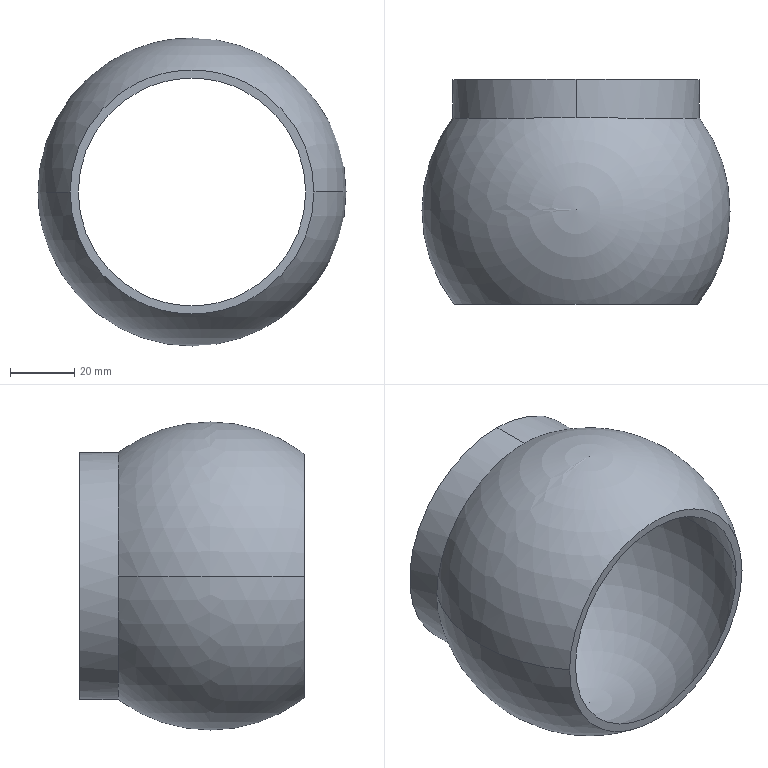Part | SolidWorks | features Revolution 1, Shell 1 | 1 solid | 10 faces | box 96 x 70 x 96 mm | volume 39871 mm3 | sphere 4 | cylinder 4 | plane 2 | commonest cylinder face diameters 73 x2 77 x2
STEP:
#1=CARTESIAN_POINT('',(35.433,-70.,0.));
#2=VERTEX_POINT('',#1);
#3=CARTESIAN_POINT('',(-35.433,-70.,0.));
#4=VERTEX_POINT('',#3);
#5=CARTESIAN_POINT('',(0.,-70.,0.));
#6=DIRECTION('',(0.,1.,0.));
#7=DIRECTION('',(0.,0.,-1.));
#8=AXIS2_PLACEMENT_3D('',#5,#6,#7);
#9=CIRCLE('',#8,35.433);
#10=EDGE_CURVE('',#2,#4,#9,.T.);
#11=ORIENTED_EDGE('',*,*,#10,.F.);
#12=CARTESIAN_POINT('',(36.5,-12.671,0.));
#13=VERTEX_POINT('',#12);
#14=CARTESIAN_POINT('',(0.,-40.666,0.));
#15=DIRECTION('',(0.,0.,1.));
#16=DIRECTION('',(1.,0.,0.));
#17=AXIS2_PLACEMENT_3D('',#14,#15,#16);
#18=CIRCLE('',#17,46.);
#19=EDGE_CURVE('',#2,#13,#18,.T.);
#20=ORIENTED_EDGE('',*,*,#19,.T.);
#21=CARTESIAN_POINT('',(0.,-12.671,-36.5));
#22=VERTEX_POINT('',#21);
#23=CARTESIAN_POINT('',(0.,-12.671,0.));
#24=DIRECTION('',(0.,1.,0.));
#25=DIRECTION('',(0.,0.,-1.));
#26=AXIS2_PLACEMENT_3D('',#23,#24,#25);
#27=CIRCLE('',#26,36.5);
#28=EDGE_CURVE('',#13,#22,#27,.T.);
#29=ORIENTED_EDGE('',*,*,#28,.T.);
#30=CARTESIAN_POINT('',(-36.5,-12.671,0.));
#31=VERTEX_POINT('',#30);
#32=CARTESIAN_POINT('',(0.,-12.671,0.));
#33=DIRECTION('',(0.,1.,0.));
#34=DIRECTION('',(0.,0.,-1.));
#35=AXIS2_PLACEMENT_3D('',#32,#33,#34);
#36=CIRCLE('',#35,36.5);
#37=EDGE_CURVE('',#22,#31,#36,.T.);
#38=ORIENTED_EDGE('',*,*,#37,.T.);
#39=CARTESIAN_POINT('',(0.,-40.666,0.));
#40=DIRECTION('',(0.,0.,-1.));
#41=DIRECTION('',(-1.,0.,0.));
#42=AXIS2_PLACEMENT_3D('',#39,#40,#41);
#43=CIRCLE('',#42,46.);
#44=EDGE_CURVE('',#4,#31,#43,.T.);
#45=ORIENTED_EDGE('',*,*,#44,.F.);
#46=EDGE_LOOP('',(#11,#20,#29,#38,#45));
#47=FACE_OUTER_BOUND('',#46,.T.);
#48=CARTESIAN_POINT('',(0.,-40.666,0.));
#49=DIRECTION('',(0.,0.,1.));
#50=DIRECTION('',(-1.,0.,0.));
#51=AXIS2_PLACEMENT_3D('',#48,#49,#50);
#52=SPHERICAL_SURFACE('',#51,46.);
#53=ADVANCED_FACE('',(#47),#52,.F.);
#54=ORIENTED_EDGE('',*,*,#37,.F.);
#55=CARTESIAN_POINT('',(0.,0.,-36.5));
#56=VERTEX_POINT('',#55);
#57=CARTESIAN_POINT('',(0.,0.,-36.5));
#58=DIRECTION('',(0.,1.,0.));
#59=VECTOR('',#58,1000.);
#60=LINE('',#57,#59);
#61=EDGE_CURVE('',#22,#56,#60,.T.);
#62=ORIENTED_EDGE('',*,*,#61,.T.);
#63=CARTESIAN_POINT('',(0.,0.,36.5));
#64=VERTEX_POINT('',#63);
#65=CARTESIAN_POINT('',(0.,0.,0.));
#66=DIRECTION('',(0.,1.,0.));
#67=DIRECTION('',(0.,0.,1.));
#68=AXIS2_PLACEMENT_3D('',#65,#66,#67);
#69=CIRCLE('',#68,36.5);
#70=EDGE_CURVE('',#56,#64,#69,.T.);
#71=ORIENTED_EDGE('',*,*,#70,.T.);
#72=CARTESIAN_POINT('',(0.,-12.671,36.5));
#73=VERTEX_POINT('',#72);
#74=CARTESIAN_POINT('',(0.,0.,36.5));
#75=DIRECTION('',(0.,1.,0.));
#76=VECTOR('',#75,1000.);
#77=LINE('',#74,#76);
#78=EDGE_CURVE('',#73,#64,#77,.T.);
#79=ORIENTED_EDGE('',*,*,#78,.F.);
#80=CARTESIAN_POINT('',(0.,-12.671,0.));
#81=DIRECTION('',(0.,1.,0.));
#82=DIRECTION('',(0.,0.,-1.));
#83=AXIS2_PLACEMENT_3D('',#80,#81,#82);
#84=CIRCLE('',#83,36.5);
#85=EDGE_CURVE('',#31,#73,#84,.T.);
#86=ORIENTED_EDGE('',*,*,#85,.F.);
#87=EDGE_LOOP('',(#54,#62,#71,#79,#86));
#88=FACE_OUTER_BOUND('',#87,.T.);
#89=CARTESIAN_POINT('',(0.,0.,0.));
#90=DIRECTION('',(0.,1.,0.));
#91=DIRECTION('',(0.,0.,1.));
#92=AXIS2_PLACEMENT_3D('',#89,#90,#91);
#93=CYLINDRICAL_SURFACE('',#92,36.5);
#94=ADVANCED_FACE('',(#88),#93,.F.);
#95=CARTESIAN_POINT('',(-37.994,-70.,0.));
#96=VERTEX_POINT('',#95);
#97=CARTESIAN_POINT('',(37.994,-70.,0.));
#98=VERTEX_POINT('',#97);
#99=CARTESIAN_POINT('',(0.,-70.,0.));
#100=DIRECTION('',(0.,1.,0.));
#101=DIRECTION('',(0.,0.,1.));
#102=AXIS2_PLACEMENT_3D('',#99,#100,#101);
#103=CIRCLE('',#102,37.994);
#104=EDGE_CURVE('',#96,#98,#103,.T.);
#105=ORIENTED_EDGE('',*,*,#104,.T.);
#106=CARTESIAN_POINT('',(38.5,-12.,0.));
#107=VERTEX_POINT('',#106);
#108=CARTESIAN_POINT('',(0.,-40.666,0.));
#109=DIRECTION('',(0.,0.,1.));
#110=DIRECTION('',(1.,0.,0.));
#111=AXIS2_PLACEMENT_3D('',#108,#109,#110);
#112=CIRCLE('',#111,48.);
#113=EDGE_CURVE('',#98,#107,#112,.T.);
#114=ORIENTED_EDGE('',*,*,#113,.T.);
#115=CARTESIAN_POINT('',(0.,-12.,38.5));
#116=VERTEX_POINT('',#115);
#117=CARTESIAN_POINT('',(0.,-12.,0.));
#118=DIRECTION('',(0.,1.,0.));
#119=DIRECTION('',(0.,0.,1.));
#120=AXIS2_PLACEMENT_3D('',#117,#118,#119);
#121=CIRCLE('',#120,38.5);
#122=EDGE_CURVE('',#116,#107,#121,.T.);
#123=ORIENTED_EDGE('',*,*,#122,.F.);
#124=CARTESIAN_POINT('',(-38.5,-12.,0.));
#125=VERTEX_POINT('',#124);
#126=CARTESIAN_POINT('',(0.,-12.,0.));
#127=DIRECTION('',(0.,1.,0.));
#128=DIRECTION('',(0.,0.,1.));
#129=AXIS2_PLACEMENT_3D('',#126,#127,#128);
#130=CIRCLE('',#129,38.5);
#131=EDGE_CURVE('',#125,#116,#130,.T.);
#132=ORIENTED_EDGE('',*,*,#131,.F.);
#133=CARTESIAN_POINT('',(0.,-40.666,0.));
#134=DIRECTION('',(0.,0.,-1.));
#135=DIRECTION('',(-1.,0.,0.));
#136=AXIS2_PLACEMENT_3D('',#133,#134,#135);
#137=CIRCLE('',#136,48.);
#138=EDGE_CURVE('',#96,#125,#137,.T.);
#139=ORIENTED_EDGE('',*,*,#138,.F.);
#140=EDGE_LOOP('',(#105,#114,#123,#132,#139));
#141=FACE_OUTER_BOUND('',#140,.T.);
#142=CARTESIAN_POINT('',(0.,-40.666,0.));
#143=DIRECTION('',(0.,0.,1.));
#144=DIRECTION('',(-1.,0.,0.));
#145=AXIS2_PLACEMENT_3D('',#142,#143,#144);
#146=SPHERICAL_SURFACE('',#145,48.);
#147=ADVANCED_FACE('',(#141),#146,.T.);
#148=ORIENTED_EDGE('',*,*,#122,.T.);
#149=CARTESIAN_POINT('',(0.,-12.,-38.5));
#150=VERTEX_POINT('',#149);
#151=CARTESIAN_POINT('',(0.,-12.,0.));
#152=DIRECTION('',(0.,1.,0.));
#153=DIRECTION('',(0.,0.,1.));
#154=AXIS2_PLACEMENT_3D('',#151,#152,#153);
#155=CIRCLE('',#154,38.5);
#156=EDGE_CURVE('',#107,#150,#155,.T.);
#157=ORIENTED_EDGE('',*,*,#156,.T.);
#158=CARTESIAN_POINT('',(0.,0.,-38.5));
#159=VERTEX_POINT('',#158);
#160=CARTESIAN_POINT('',(0.,0.,-38.5));
#161=DIRECTION('',(0.,1.,0.));
#162=VECTOR('',#161,1000.);
#163=LINE('',#160,#162);
#164=EDGE_CURVE('',#150,#159,#163,.T.);
#165=ORIENTED_EDGE('',*,*,#164,.T.);
#166=CARTESIAN_POINT('',(0.,0.,38.5));
#167=VERTEX_POINT('',#166);
#168=CARTESIAN_POINT('',(0.,0.,0.));
#169=DIRECTION('',(0.,1.,0.));
#170=DIRECTION('',(0.,0.,1.));
#171=AXIS2_PLACEMENT_3D('',#168,#169,#170);
#172=CIRCLE('',#171,38.5);
#173=EDGE_CURVE('',#167,#159,#172,.T.);
#174=ORIENTED_EDGE('',*,*,#173,.F.);
#175=CARTESIAN_POINT('',(0.,0.,38.5));
#176=DIRECTION('',(0.,1.,0.));
#177=VECTOR('',#176,1000.);
#178=LINE('',#175,#177);
#179=EDGE_CURVE('',#116,#167,#178,.T.);
#180=ORIENTED_EDGE('',*,*,#179,.F.);
#181=EDGE_LOOP('',(#148,#157,#165,#174,#180));
#182=FACE_OUTER_BOUND('',#181,.T.);
#183=CARTESIAN_POINT('',(0.,0.,0.));
#184=DIRECTION('',(0.,1.,0.));
#185=DIRECTION('',(0.,0.,1.));
#186=AXIS2_PLACEMENT_3D('',#183,#184,#185);
#187=CYLINDRICAL_SURFACE('',#186,38.5);
#188=ADVANCED_FACE('',(#182),#187,.T.);
#189=ORIENTED_EDGE('',*,*,#104,.F.);
#190=CARTESIAN_POINT('',(0.,-70.,0.));
#191=DIRECTION('',(0.,1.,0.));
#192=DIRECTION('',(0.,0.,1.));
#193=AXIS2_PLACEMENT_3D('',#190,#191,#192);
#194=CIRCLE('',#193,37.994);
#195=EDGE_CURVE('',#98,#96,#194,.T.);
#196=ORIENTED_EDGE('',*,*,#195,.F.);
#197=EDGE_LOOP('',(#189,#196));
#198=FACE_OUTER_BOUND('',#197,.T.);
#199=CARTESIAN_POINT('',(0.,-70.,0.));
#200=DIRECTION('',(0.,1.,0.));
#201=DIRECTION('',(0.,0.,-1.));
#202=AXIS2_PLACEMENT_3D('',#199,#200,#201);
#203=CIRCLE('',#202,35.433);
#204=EDGE_CURVE('',#4,#2,#203,.T.);
#205=ORIENTED_EDGE('',*,*,#204,.T.);
#206=ORIENTED_EDGE('',*,*,#10,.T.);
#207=EDGE_LOOP('',(#205,#206));
#208=FACE_BOUND('',#207,.T.);
#209=CARTESIAN_POINT('',(-37.994,-70.,0.));
#210=DIRECTION('',(0.,-1.,0.));
#211=DIRECTION('',(0.,0.,-1.));
#212=AXIS2_PLACEMENT_3D('',#209,#210,#211);
#213=PLANE('',#212);
#214=ADVANCED_FACE('',(#198,#208),#213,.T.);
#215=CARTESIAN_POINT('',(0.,0.,0.));
#216=DIRECTION('',(0.,1.,0.));
#217=DIRECTION('',(0.,0.,1.));
#218=AXIS2_PLACEMENT_3D('',#215,#216,#217);
#219=CIRCLE('',#218,36.5);
#220=EDGE_CURVE('',#64,#56,#219,.T.);
#221=ORIENTED_EDGE('',*,*,#220,.F.);
#222=ORIENTED_EDGE('',*,*,#70,.F.);
#223=EDGE_LOOP('',(#221,#222));
#224=FACE_BOUND('',#223,.T.);
#225=ORIENTED_EDGE('',*,*,#173,.T.);
#226=CARTESIAN_POINT('',(0.,0.,0.));
#227=DIRECTION('',(0.,1.,0.));
#228=DIRECTION('',(0.,0.,1.));
#229=AXIS2_PLACEMENT_3D('',#226,#227,#228);
#230=CIRCLE('',#229,38.5);
#231=EDGE_CURVE('',#159,#167,#230,.T.);
#232=ORIENTED_EDGE('',*,*,#231,.T.);
#233=EDGE_LOOP('',(#225,#232));
#234=FACE_OUTER_BOUND('',#233,.T.);
#235=CARTESIAN_POINT('',(0.,0.,0.));
#236=DIRECTION('',(0.,1.,0.));
#237=DIRECTION('',(0.,0.,1.));
#238=AXIS2_PLACEMENT_3D('',#235,#236,#237);
#239=PLANE('',#238);
#240=ADVANCED_FACE('',(#224,#234),#239,.T.);
#241=ORIENTED_EDGE('',*,*,#164,.F.);
#242=CARTESIAN_POINT('',(0.,-12.,0.));
#243=DIRECTION('',(0.,1.,0.));
#244=DIRECTION('',(0.,0.,1.));
#245=AXIS2_PLACEMENT_3D('',#242,#243,#244);
#246=CIRCLE('',#245,38.5);
#247=EDGE_CURVE('',#150,#125,#246,.T.);
#248=ORIENTED_EDGE('',*,*,#247,.T.);
#249=ORIENTED_EDGE('',*,*,#131,.T.);
#250=ORIENTED_EDGE('',*,*,#179,.T.);
#251=ORIENTED_EDGE('',*,*,#231,.F.);
#252=EDGE_LOOP('',(#241,#248,#249,#250,#251));
#253=FACE_OUTER_BOUND('',#252,.T.);
#254=CARTESIAN_POINT('',(0.,0.,0.));
#255=DIRECTION('',(0.,1.,0.));
#256=DIRECTION('',(0.,0.,1.));
#257=AXIS2_PLACEMENT_3D('',#254,#255,#256);
#258=CYLINDRICAL_SURFACE('',#257,38.5);
#259=ADVANCED_FACE('',(#253),#258,.T.);
#260=ORIENTED_EDGE('',*,*,#113,.F.);
#261=ORIENTED_EDGE('',*,*,#195,.T.);
#262=ORIENTED_EDGE('',*,*,#138,.T.);
#263=ORIENTED_EDGE('',*,*,#247,.F.);
#264=ORIENTED_EDGE('',*,*,#156,.F.);
#265=EDGE_LOOP('',(#260,#261,#262,#263,#264));
#266=FACE_OUTER_BOUND('',#265,.T.);
#267=CARTESIAN_POINT('',(0.,-40.666,0.));
#268=DIRECTION('',(0.,0.,1.));
#269=DIRECTION('',(-1.,0.,0.));
#270=AXIS2_PLACEMENT_3D('',#267,#268,#269);
#271=SPHERICAL_SURFACE('',#270,48.);
#272=ADVANCED_FACE('',(#266),#271,.T.);
#273=ORIENTED_EDGE('',*,*,#61,.F.);
#274=ORIENTED_EDGE('',*,*,#28,.F.);
#275=CARTESIAN_POINT('',(0.,-12.671,0.));
#276=DIRECTION('',(0.,1.,0.));
#277=DIRECTION('',(0.,0.,-1.));
#278=AXIS2_PLACEMENT_3D('',#275,#276,#277);
#279=CIRCLE('',#278,36.5);
#280=EDGE_CURVE('',#73,#13,#279,.T.);
#281=ORIENTED_EDGE('',*,*,#280,.F.);
#282=ORIENTED_EDGE('',*,*,#78,.T.);
#283=ORIENTED_EDGE('',*,*,#220,.T.);
#284=EDGE_LOOP('',(#273,#274,#281,#282,#283));
#285=FACE_OUTER_BOUND('',#284,.T.);
#286=CARTESIAN_POINT('',(0.,0.,0.));
#287=DIRECTION('',(0.,1.,0.));
#288=DIRECTION('',(0.,0.,1.));
#289=AXIS2_PLACEMENT_3D('',#286,#287,#288);
#290=CYLINDRICAL_SURFACE('',#289,36.5);
#291=ADVANCED_FACE('',(#285),#290,.F.);
#292=ORIENTED_EDGE('',*,*,#19,.F.);
#293=ORIENTED_EDGE('',*,*,#204,.F.);
#294=ORIENTED_EDGE('',*,*,#44,.T.);
#295=ORIENTED_EDGE('',*,*,#85,.T.);
#296=ORIENTED_EDGE('',*,*,#280,.T.);
#297=EDGE_LOOP('',(#292,#293,#294,#295,#296));
#298=FACE_OUTER_BOUND('',#297,.T.);
#299=CARTESIAN_POINT('',(0.,-40.666,0.));
#300=DIRECTION('',(0.,0.,1.));
#301=DIRECTION('',(-1.,0.,0.));
#302=AXIS2_PLACEMENT_3D('',#299,#300,#301);
#303=SPHERICAL_SURFACE('',#302,46.);
#304=ADVANCED_FACE('',(#298),#303,.F.);
#305=CLOSED_SHELL('',(#53,#94,#147,#188,#214,#240,#259,#272,#291,#304));
#306=MANIFOLD_SOLID_BREP('',#305);
#307=CARTESIAN_POINT('',(0.,0.,0.));
#308=DIRECTION('',(0.,0.,1.));
#309=DIRECTION('',(1.,0.,0.));
#310=AXIS2_PLACEMENT_3D('',#307,#308,#309);
#311=(LENGTH_UNIT()NAMED_UNIT(*)SI_UNIT(.MILLI.,.METRE.));
#312=UNCERTAINTY_MEASURE_WITH_UNIT(LENGTH_MEASURE(0.00001),#311,'','');
#313=(NAMED_UNIT(*)PLANE_ANGLE_UNIT()SI_UNIT($,.RADIAN.));
#314=(NAMED_UNIT(*)SI_UNIT($,.STERADIAN.)SOLID_ANGLE_UNIT());
#315=(GEOMETRIC_REPRESENTATION_CONTEXT(3)GLOBAL_UNCERTAINTY_ASSIGNED_CONTEXT((#312))GLOBAL_UNIT_ASSIGNED_CONTEXT((#311,#313,#314))REPRESENTATION_CONTEXT('',''));
#316=ADVANCED_BREP_SHAPE_REPRESENTATION('',(#306,#310),#315);